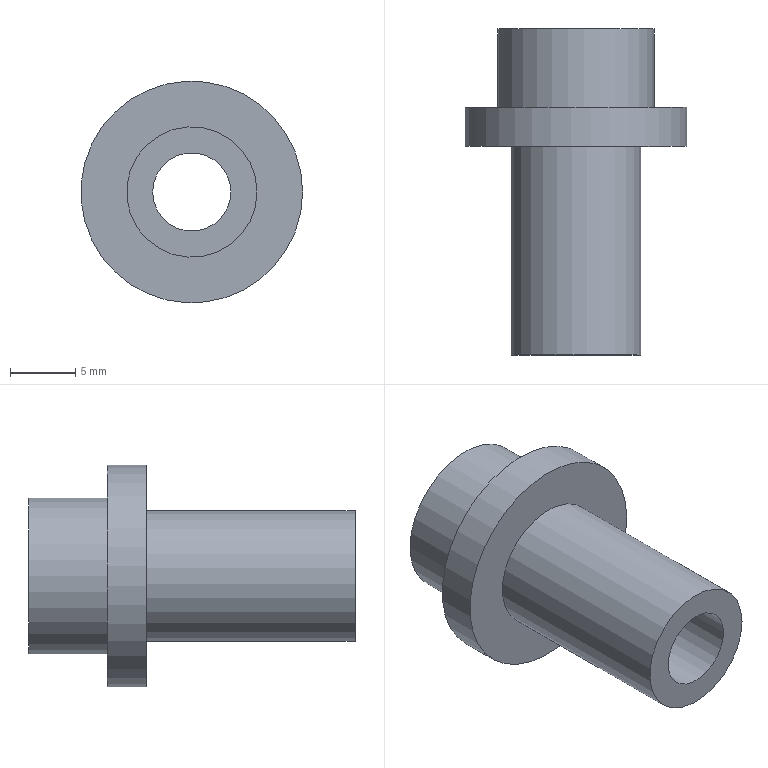Part | STEP file | 1-61.2 | 1 solid | 8 faces | box 17 x 25 x 17 mm | volume 1909 mm3 | cylinder 4 | plane 4 | commonest cylinder face diameters 6 x1 10 x1 12 x1 17 x1
STEP:
#1=CARTESIAN_POINT('',(0.,0.,0.));
#2=DIRECTION('',(0.,0.,1.));
#3=DIRECTION('',(1.,0.,0.));
#4=AXIS2_PLACEMENT_3D('',#1,#2,#3);
#5=CARTESIAN_POINT('',(8.5,0.,0.));
#6=VERTEX_POINT('',#5);
#7=CARTESIAN_POINT('',(8.5,3.,0.));
#8=VERTEX_POINT('',#7);
#9=CARTESIAN_POINT('',(8.5,0.,0.));
#10=DIRECTION('',(0.,1.,0.));
#11=VECTOR('',#10,1.);
#12=LINE('',#9,#11);
#13=CARTESIAN_POINT('',(0.,0.,0.));
#14=DIRECTION('',(0.,1.,0.));
#15=DIRECTION('',(1.,0.,0.));
#16=AXIS2_PLACEMENT_3D('',#13,#14,#15);
#17=CYLINDRICAL_SURFACE('',#16,8.5);
#18=CARTESIAN_POINT('',(6.283,0.));
#19=DIRECTION('',(0.,1.));
#20=VECTOR('',#19,1.);
#21=LINE('',#18,#20);
#22=(GEOMETRIC_REPRESENTATION_CONTEXT(2)PARAMETRIC_REPRESENTATION_CONTEXT()REPRESENTATION_CONTEXT('',''));
#23=DEFINITIONAL_REPRESENTATION('',(#21),#22);
#24=PCURVE('',#17,#23);
#25=CARTESIAN_POINT('',(0.,0.));
#26=DIRECTION('',(0.,1.));
#27=VECTOR('',#26,1.);
#28=LINE('',#25,#27);
#29=(GEOMETRIC_REPRESENTATION_CONTEXT(2)PARAMETRIC_REPRESENTATION_CONTEXT()REPRESENTATION_CONTEXT('',''));
#30=DEFINITIONAL_REPRESENTATION('',(#28),#29);
#31=PCURVE('',#17,#30);
#32=SEAM_CURVE('',#12,(#24,#31),.PCURVE_S1.);
#33=EDGE_CURVE('',#6,#8,#32,.T.);
#34=ORIENTED_EDGE('',*,*,#33,.T.);
#35=CARTESIAN_POINT('',(0.,3.,0.));
#36=DIRECTION('',(0.,-1.,0.));
#37=DIRECTION('',(1.,0.,0.));
#38=AXIS2_PLACEMENT_3D('',#35,#36,#37);
#39=CIRCLE('',#38,8.5);
#40=CARTESIAN_POINT('',(6.283,3.));
#41=DIRECTION('',(-1.,0.));
#42=VECTOR('',#41,1.);
#43=LINE('',#40,#42);
#44=(GEOMETRIC_REPRESENTATION_CONTEXT(2)PARAMETRIC_REPRESENTATION_CONTEXT()REPRESENTATION_CONTEXT('',''));
#45=DEFINITIONAL_REPRESENTATION('',(#43),#44);
#46=PCURVE('',#17,#45);
#47=CARTESIAN_POINT('',(-2.278,3.,0.));
#48=DIRECTION('',(0.,-1.,0.));
#49=DIRECTION('',(1.,0.,0.));
#50=AXIS2_PLACEMENT_3D('',#47,#48,#49);
#51=PLANE('',#50);
#52=CARTESIAN_POINT('',(2.278,0.));
#53=DIRECTION('',(1.,0.));
#54=AXIS2_PLACEMENT_2D('',#52,#53);
#55=CIRCLE('',#54,8.5);
#56=(GEOMETRIC_REPRESENTATION_CONTEXT(2)PARAMETRIC_REPRESENTATION_CONTEXT()REPRESENTATION_CONTEXT('',''));
#57=DEFINITIONAL_REPRESENTATION('',(#55),#56);
#58=PCURVE('',#51,#57);
#59=SURFACE_CURVE('',#39,(#46,#58),.PCURVE_S1.);
#60=EDGE_CURVE('',#8,#8,#59,.T.);
#61=ORIENTED_EDGE('',*,*,#60,.T.);
#62=ORIENTED_EDGE('',*,*,#33,.F.);
#63=CARTESIAN_POINT('',(0.,0.,0.));
#64=DIRECTION('',(0.,-1.,0.));
#65=DIRECTION('',(1.,0.,0.));
#66=AXIS2_PLACEMENT_3D('',#63,#64,#65);
#67=CIRCLE('',#66,8.5);
#68=CARTESIAN_POINT('',(6.283,0.));
#69=DIRECTION('',(-1.,0.));
#70=VECTOR('',#69,1.);
#71=LINE('',#68,#70);
#72=(GEOMETRIC_REPRESENTATION_CONTEXT(2)PARAMETRIC_REPRESENTATION_CONTEXT()REPRESENTATION_CONTEXT('',''));
#73=DEFINITIONAL_REPRESENTATION('',(#71),#72);
#74=PCURVE('',#17,#73);
#75=CARTESIAN_POINT('',(-2.278,0.,0.));
#76=DIRECTION('',(0.,-1.,0.));
#77=DIRECTION('',(1.,0.,0.));
#78=AXIS2_PLACEMENT_3D('',#75,#76,#77);
#79=PLANE('',#78);
#80=CARTESIAN_POINT('',(2.278,0.));
#81=DIRECTION('',(1.,0.));
#82=AXIS2_PLACEMENT_2D('',#80,#81);
#83=CIRCLE('',#82,8.5);
#84=(GEOMETRIC_REPRESENTATION_CONTEXT(2)PARAMETRIC_REPRESENTATION_CONTEXT()REPRESENTATION_CONTEXT('',''));
#85=DEFINITIONAL_REPRESENTATION('',(#83),#84);
#86=PCURVE('',#79,#85);
#87=SURFACE_CURVE('',#67,(#74,#86),.PCURVE_S1.);
#88=EDGE_CURVE('',#6,#6,#87,.T.);
#89=ORIENTED_EDGE('',*,*,#88,.F.);
#90=EDGE_LOOP('',(#34,#61,#62,#89));
#91=FACE_BOUND('',#90,.T.);
#92=ADVANCED_FACE('',(#91),#17,.T.);
#93=CARTESIAN_POINT('',(3.,9.,0.));
#94=VERTEX_POINT('',#93);
#95=CARTESIAN_POINT('',(0.,9.,0.));
#96=DIRECTION('',(0.,1.,0.));
#97=DIRECTION('',(1.,0.,0.));
#98=AXIS2_PLACEMENT_3D('',#95,#96,#97);
#99=CIRCLE('',#98,3.);
#100=CARTESIAN_POINT('',(0.,-16.,0.));
#101=DIRECTION('',(0.,1.,0.));
#102=DIRECTION('',(1.,0.,0.));
#103=AXIS2_PLACEMENT_3D('',#100,#101,#102);
#104=CYLINDRICAL_SURFACE('',#103,3.);
#105=CARTESIAN_POINT('',(0.,25.));
#106=DIRECTION('',(1.,0.));
#107=VECTOR('',#106,1.);
#108=LINE('',#105,#107);
#109=(GEOMETRIC_REPRESENTATION_CONTEXT(2)PARAMETRIC_REPRESENTATION_CONTEXT()REPRESENTATION_CONTEXT('',''));
#110=DEFINITIONAL_REPRESENTATION('',(#108),#109);
#111=PCURVE('',#104,#110);
#112=CARTESIAN_POINT('',(-1.608,9.,0.));
#113=DIRECTION('',(0.,-1.,0.));
#114=DIRECTION('',(1.,0.,0.));
#115=AXIS2_PLACEMENT_3D('',#112,#113,#114);
#116=PLANE('',#115);
#117=CARTESIAN_POINT('',(4.608,0.));
#118=CARTESIAN_POINT('',(4.608,-5.196));
#119=CARTESIAN_POINT('',(0.1077,-2.598));
#120=CARTESIAN_POINT('',(-4.392,0.));
#121=CARTESIAN_POINT('',(0.1077,2.598));
#122=CARTESIAN_POINT('',(4.608,5.196));
#123=CARTESIAN_POINT('',(4.608,0.));
#124=(BOUNDED_CURVE()B_SPLINE_CURVE(2,(#117,#118,#119,#120,#121,#122,#123),.UNSPECIFIED.,.T.,.F.)B_SPLINE_CURVE_WITH_KNOTS((1,2,2,2,2,1),(-2.094,0.,2.094,4.189,6.283,8.378),.UNSPECIFIED.)CURVE()GEOMETRIC_REPRESENTATION_ITEM()RATIONAL_B_SPLINE_CURVE((1.,0.5,1.,0.5,1.,0.5,1.))REPRESENTATION_ITEM(''));
#125=(GEOMETRIC_REPRESENTATION_CONTEXT(2)PARAMETRIC_REPRESENTATION_CONTEXT()REPRESENTATION_CONTEXT('',''));
#126=DEFINITIONAL_REPRESENTATION('',(#124),#125);
#127=PCURVE('',#116,#126);
#128=SURFACE_CURVE('',#99,(#111,#127),.PCURVE_S1.);
#129=EDGE_CURVE('',#94,#94,#128,.T.);
#130=ORIENTED_EDGE('',*,*,#129,.F.);
#131=CARTESIAN_POINT('',(3.,-16.,0.));
#132=VERTEX_POINT('',#131);
#133=CARTESIAN_POINT('',(3.,9.,0.));
#134=DIRECTION('',(0.,-1.,0.));
#135=VECTOR('',#134,1.);
#136=LINE('',#133,#135);
#137=CARTESIAN_POINT('',(0.,25.));
#138=DIRECTION('',(0.,-1.));
#139=VECTOR('',#138,1.);
#140=LINE('',#137,#139);
#141=(GEOMETRIC_REPRESENTATION_CONTEXT(2)PARAMETRIC_REPRESENTATION_CONTEXT()REPRESENTATION_CONTEXT('',''));
#142=DEFINITIONAL_REPRESENTATION('',(#140),#141);
#143=PCURVE('',#104,#142);
#144=CARTESIAN_POINT('',(6.283,25.));
#145=DIRECTION('',(0.,-1.));
#146=VECTOR('',#145,1.);
#147=LINE('',#144,#146);
#148=(GEOMETRIC_REPRESENTATION_CONTEXT(2)PARAMETRIC_REPRESENTATION_CONTEXT()REPRESENTATION_CONTEXT('',''));
#149=DEFINITIONAL_REPRESENTATION('',(#147),#148);
#150=PCURVE('',#104,#149);
#151=SEAM_CURVE('',#136,(#143,#150),.PCURVE_S1.);
#152=EDGE_CURVE('',#94,#132,#151,.T.);
#153=ORIENTED_EDGE('',*,*,#152,.T.);
#154=CARTESIAN_POINT('',(0.,-16.,0.));
#155=DIRECTION('',(0.,1.,0.));
#156=DIRECTION('',(1.,0.,0.));
#157=AXIS2_PLACEMENT_3D('',#154,#155,#156);
#158=CIRCLE('',#157,3.);
#159=CARTESIAN_POINT('',(0.,0.));
#160=DIRECTION('',(1.,0.));
#161=VECTOR('',#160,1.);
#162=LINE('',#159,#161);
#163=(GEOMETRIC_REPRESENTATION_CONTEXT(2)PARAMETRIC_REPRESENTATION_CONTEXT()REPRESENTATION_CONTEXT('',''));
#164=DEFINITIONAL_REPRESENTATION('',(#162),#163);
#165=PCURVE('',#104,#164);
#166=CARTESIAN_POINT('',(-1.34,-16.,0.));
#167=DIRECTION('',(0.,-1.,0.));
#168=DIRECTION('',(1.,0.,0.));
#169=AXIS2_PLACEMENT_3D('',#166,#167,#168);
#170=PLANE('',#169);
#171=CARTESIAN_POINT('',(4.34,0.));
#172=CARTESIAN_POINT('',(4.34,-5.196));
#173=CARTESIAN_POINT('',(-0.1603,-2.598));
#174=CARTESIAN_POINT('',(-4.66,0.));
#175=CARTESIAN_POINT('',(-0.1603,2.598));
#176=CARTESIAN_POINT('',(4.34,5.196));
#177=CARTESIAN_POINT('',(4.34,0.));
#178=(BOUNDED_CURVE()B_SPLINE_CURVE(2,(#171,#172,#173,#174,#175,#176,#177),.UNSPECIFIED.,.T.,.F.)B_SPLINE_CURVE_WITH_KNOTS((1,2,2,2,2,1),(-2.094,0.,2.094,4.189,6.283,8.378),.UNSPECIFIED.)CURVE()GEOMETRIC_REPRESENTATION_ITEM()RATIONAL_B_SPLINE_CURVE((1.,0.5,1.,0.5,1.,0.5,1.))REPRESENTATION_ITEM(''));
#179=(GEOMETRIC_REPRESENTATION_CONTEXT(2)PARAMETRIC_REPRESENTATION_CONTEXT()REPRESENTATION_CONTEXT('',''));
#180=DEFINITIONAL_REPRESENTATION('',(#178),#179);
#181=PCURVE('',#170,#180);
#182=SURFACE_CURVE('',#158,(#165,#181),.PCURVE_S1.);
#183=EDGE_CURVE('',#132,#132,#182,.T.);
#184=ORIENTED_EDGE('',*,*,#183,.T.);
#185=ORIENTED_EDGE('',*,*,#152,.F.);
#186=EDGE_LOOP('',(#130,#153,#184,#185));
#187=FACE_BOUND('',#186,.F.);
#188=ADVANCED_FACE('',(#187),#104,.F.);
#189=ORIENTED_EDGE('',*,*,#60,.T.);
#190=EDGE_LOOP('',(#189));
#191=FACE_BOUND('',#190,.F.);
#192=CARTESIAN_POINT('',(6.,3.,0.));
#193=VERTEX_POINT('',#192);
#194=CARTESIAN_POINT('',(0.,3.,0.));
#195=DIRECTION('',(0.,-1.,0.));
#196=DIRECTION('',(1.,0.,0.));
#197=AXIS2_PLACEMENT_3D('',#194,#195,#196);
#198=CIRCLE('',#197,6.);
#199=CARTESIAN_POINT('',(2.278,0.));
#200=DIRECTION('',(1.,0.));
#201=AXIS2_PLACEMENT_2D('',#199,#200);
#202=CIRCLE('',#201,6.);
#203=(GEOMETRIC_REPRESENTATION_CONTEXT(2)PARAMETRIC_REPRESENTATION_CONTEXT()REPRESENTATION_CONTEXT('',''));
#204=DEFINITIONAL_REPRESENTATION('',(#202),#203);
#205=PCURVE('',#51,#204);
#206=CARTESIAN_POINT('',(0.,3.,0.));
#207=DIRECTION('',(0.,1.,0.));
#208=DIRECTION('',(1.,0.,0.));
#209=AXIS2_PLACEMENT_3D('',#206,#207,#208);
#210=CYLINDRICAL_SURFACE('',#209,6.);
#211=CARTESIAN_POINT('',(6.283,0.));
#212=DIRECTION('',(-1.,0.));
#213=VECTOR('',#212,1.);
#214=LINE('',#211,#213);
#215=(GEOMETRIC_REPRESENTATION_CONTEXT(2)PARAMETRIC_REPRESENTATION_CONTEXT()REPRESENTATION_CONTEXT('',''));
#216=DEFINITIONAL_REPRESENTATION('',(#214),#215);
#217=PCURVE('',#210,#216);
#218=SURFACE_CURVE('',#198,(#205,#217),.PCURVE_S1.);
#219=EDGE_CURVE('',#193,#193,#218,.T.);
#220=ORIENTED_EDGE('',*,*,#219,.F.);
#221=EDGE_LOOP('',(#220));
#222=FACE_BOUND('',#221,.F.);
#223=ADVANCED_FACE('',(#191,#222),#51,.F.);
#224=CARTESIAN_POINT('',(6.,9.,0.));
#225=VERTEX_POINT('',#224);
#226=CARTESIAN_POINT('',(6.,3.,0.));
#227=DIRECTION('',(0.,1.,0.));
#228=VECTOR('',#227,1.);
#229=LINE('',#226,#228);
#230=CARTESIAN_POINT('',(6.283,0.));
#231=DIRECTION('',(0.,1.));
#232=VECTOR('',#231,1.);
#233=LINE('',#230,#232);
#234=(GEOMETRIC_REPRESENTATION_CONTEXT(2)PARAMETRIC_REPRESENTATION_CONTEXT()REPRESENTATION_CONTEXT('',''));
#235=DEFINITIONAL_REPRESENTATION('',(#233),#234);
#236=PCURVE('',#210,#235);
#237=CARTESIAN_POINT('',(0.,0.));
#238=DIRECTION('',(0.,1.));
#239=VECTOR('',#238,1.);
#240=LINE('',#237,#239);
#241=(GEOMETRIC_REPRESENTATION_CONTEXT(2)PARAMETRIC_REPRESENTATION_CONTEXT()REPRESENTATION_CONTEXT('',''));
#242=DEFINITIONAL_REPRESENTATION('',(#240),#241);
#243=PCURVE('',#210,#242);
#244=SEAM_CURVE('',#229,(#236,#243),.PCURVE_S1.);
#245=EDGE_CURVE('',#193,#225,#244,.T.);
#246=ORIENTED_EDGE('',*,*,#245,.T.);
#247=CARTESIAN_POINT('',(0.,9.,0.));
#248=DIRECTION('',(0.,-1.,0.));
#249=DIRECTION('',(1.,0.,0.));
#250=AXIS2_PLACEMENT_3D('',#247,#248,#249);
#251=CIRCLE('',#250,6.);
#252=CARTESIAN_POINT('',(6.283,6.));
#253=DIRECTION('',(-1.,0.));
#254=VECTOR('',#253,1.);
#255=LINE('',#252,#254);
#256=(GEOMETRIC_REPRESENTATION_CONTEXT(2)PARAMETRIC_REPRESENTATION_CONTEXT()REPRESENTATION_CONTEXT('',''));
#257=DEFINITIONAL_REPRESENTATION('',(#255),#256);
#258=PCURVE('',#210,#257);
#259=CARTESIAN_POINT('',(1.608,0.));
#260=DIRECTION('',(1.,0.));
#261=AXIS2_PLACEMENT_2D('',#259,#260);
#262=CIRCLE('',#261,6.);
#263=(GEOMETRIC_REPRESENTATION_CONTEXT(2)PARAMETRIC_REPRESENTATION_CONTEXT()REPRESENTATION_CONTEXT('',''));
#264=DEFINITIONAL_REPRESENTATION('',(#262),#263);
#265=PCURVE('',#116,#264);
#266=SURFACE_CURVE('',#251,(#258,#265),.PCURVE_S1.);
#267=EDGE_CURVE('',#225,#225,#266,.T.);
#268=ORIENTED_EDGE('',*,*,#267,.T.);
#269=ORIENTED_EDGE('',*,*,#245,.F.);
#270=ORIENTED_EDGE('',*,*,#219,.F.);
#271=EDGE_LOOP('',(#246,#268,#269,#270));
#272=FACE_BOUND('',#271,.T.);
#273=ADVANCED_FACE('',(#272),#210,.T.);
#274=ORIENTED_EDGE('',*,*,#267,.T.);
#275=EDGE_LOOP('',(#274));
#276=FACE_BOUND('',#275,.F.);
#277=ORIENTED_EDGE('',*,*,#129,.T.);
#278=EDGE_LOOP('',(#277));
#279=FACE_BOUND('',#278,.F.);
#280=ADVANCED_FACE('',(#276,#279),#116,.F.);
#281=ORIENTED_EDGE('',*,*,#88,.T.);
#282=EDGE_LOOP('',(#281));
#283=FACE_BOUND('',#282,.T.);
#284=CARTESIAN_POINT('',(5.,0.,0.));
#285=VERTEX_POINT('',#284);
#286=CARTESIAN_POINT('',(0.,0.,0.));
#287=DIRECTION('',(0.,-1.,0.));
#288=DIRECTION('',(1.,0.,0.));
#289=AXIS2_PLACEMENT_3D('',#286,#287,#288);
#290=CIRCLE('',#289,5.);
#291=CARTESIAN_POINT('',(2.278,0.));
#292=DIRECTION('',(1.,0.));
#293=AXIS2_PLACEMENT_2D('',#291,#292);
#294=CIRCLE('',#293,5.);
#295=(GEOMETRIC_REPRESENTATION_CONTEXT(2)PARAMETRIC_REPRESENTATION_CONTEXT()REPRESENTATION_CONTEXT('',''));
#296=DEFINITIONAL_REPRESENTATION('',(#294),#295);
#297=PCURVE('',#79,#296);
#298=CARTESIAN_POINT('',(0.,0.,0.));
#299=DIRECTION('',(0.,-1.,0.));
#300=DIRECTION('',(1.,0.,0.));
#301=AXIS2_PLACEMENT_3D('',#298,#299,#300);
#302=CYLINDRICAL_SURFACE('',#301,5.);
#303=CARTESIAN_POINT('',(0.,0.));
#304=DIRECTION('',(1.,0.));
#305=VECTOR('',#304,1.);
#306=LINE('',#303,#305);
#307=(GEOMETRIC_REPRESENTATION_CONTEXT(2)PARAMETRIC_REPRESENTATION_CONTEXT()REPRESENTATION_CONTEXT('',''));
#308=DEFINITIONAL_REPRESENTATION('',(#306),#307);
#309=PCURVE('',#302,#308);
#310=SURFACE_CURVE('',#290,(#297,#309),.PCURVE_S1.);
#311=EDGE_CURVE('',#285,#285,#310,.T.);
#312=ORIENTED_EDGE('',*,*,#311,.F.);
#313=EDGE_LOOP('',(#312));
#314=FACE_BOUND('',#313,.T.);
#315=ADVANCED_FACE('',(#283,#314),#79,.T.);
#316=ORIENTED_EDGE('',*,*,#311,.T.);
#317=CARTESIAN_POINT('',(5.,-16.,0.));
#318=VERTEX_POINT('',#317);
#319=CARTESIAN_POINT('',(5.,0.,0.));
#320=DIRECTION('',(0.,-1.,0.));
#321=VECTOR('',#320,1.);
#322=LINE('',#319,#321);
#323=CARTESIAN_POINT('',(6.283,0.));
#324=DIRECTION('',(0.,1.));
#325=VECTOR('',#324,1.);
#326=LINE('',#323,#325);
#327=(GEOMETRIC_REPRESENTATION_CONTEXT(2)PARAMETRIC_REPRESENTATION_CONTEXT()REPRESENTATION_CONTEXT('',''));
#328=DEFINITIONAL_REPRESENTATION('',(#326),#327);
#329=PCURVE('',#302,#328);
#330=CARTESIAN_POINT('',(0.,0.));
#331=DIRECTION('',(0.,1.));
#332=VECTOR('',#331,1.);
#333=LINE('',#330,#332);
#334=(GEOMETRIC_REPRESENTATION_CONTEXT(2)PARAMETRIC_REPRESENTATION_CONTEXT()REPRESENTATION_CONTEXT('',''));
#335=DEFINITIONAL_REPRESENTATION('',(#333),#334);
#336=PCURVE('',#302,#335);
#337=SEAM_CURVE('',#322,(#329,#336),.PCURVE_S1.);
#338=EDGE_CURVE('',#285,#318,#337,.T.);
#339=ORIENTED_EDGE('',*,*,#338,.T.);
#340=CARTESIAN_POINT('',(0.,-16.,0.));
#341=DIRECTION('',(0.,-1.,0.));
#342=DIRECTION('',(1.,0.,0.));
#343=AXIS2_PLACEMENT_3D('',#340,#341,#342);
#344=CIRCLE('',#343,5.);
#345=CARTESIAN_POINT('',(0.,16.));
#346=DIRECTION('',(1.,0.));
#347=VECTOR('',#346,1.);
#348=LINE('',#345,#347);
#349=(GEOMETRIC_REPRESENTATION_CONTEXT(2)PARAMETRIC_REPRESENTATION_CONTEXT()REPRESENTATION_CONTEXT('',''));
#350=DEFINITIONAL_REPRESENTATION('',(#348),#349);
#351=PCURVE('',#302,#350);
#352=CARTESIAN_POINT('',(1.34,0.));
#353=DIRECTION('',(1.,0.));
#354=AXIS2_PLACEMENT_2D('',#352,#353);
#355=CIRCLE('',#354,5.);
#356=(GEOMETRIC_REPRESENTATION_CONTEXT(2)PARAMETRIC_REPRESENTATION_CONTEXT()REPRESENTATION_CONTEXT('',''));
#357=DEFINITIONAL_REPRESENTATION('',(#355),#356);
#358=PCURVE('',#170,#357);
#359=SURFACE_CURVE('',#344,(#351,#358),.PCURVE_S1.);
#360=EDGE_CURVE('',#318,#318,#359,.T.);
#361=ORIENTED_EDGE('',*,*,#360,.F.);
#362=ORIENTED_EDGE('',*,*,#338,.F.);
#363=EDGE_LOOP('',(#316,#339,#361,#362));
#364=FACE_BOUND('',#363,.T.);
#365=ADVANCED_FACE('',(#364),#302,.T.);
#366=ORIENTED_EDGE('',*,*,#360,.T.);
#367=EDGE_LOOP('',(#366));
#368=FACE_BOUND('',#367,.T.);
#369=ORIENTED_EDGE('',*,*,#183,.T.);
#370=EDGE_LOOP('',(#369));
#371=FACE_BOUND('',#370,.T.);
#372=ADVANCED_FACE('',(#368,#371),#170,.T.);
#373=CLOSED_SHELL('',(#92,#188,#223,#273,#280,#315,#365,#372));
#374=MANIFOLD_SOLID_BREP('',#373);
#375=(LENGTH_UNIT()NAMED_UNIT(*)SI_UNIT(.MILLI.,.METRE.));
#376=UNCERTAINTY_MEASURE_WITH_UNIT(LENGTH_MEASURE(0.0000001),#375,'','');
#377=(NAMED_UNIT(*)PLANE_ANGLE_UNIT()SI_UNIT($,.RADIAN.));
#378=(NAMED_UNIT(*)SI_UNIT($,.STERADIAN.)SOLID_ANGLE_UNIT());
#379=(GEOMETRIC_REPRESENTATION_CONTEXT(3)GLOBAL_UNCERTAINTY_ASSIGNED_CONTEXT((#376))GLOBAL_UNIT_ASSIGNED_CONTEXT((#375,#377,#378))REPRESENTATION_CONTEXT('',''));
#380=ADVANCED_BREP_SHAPE_REPRESENTATION('',(#4,#374),#379);